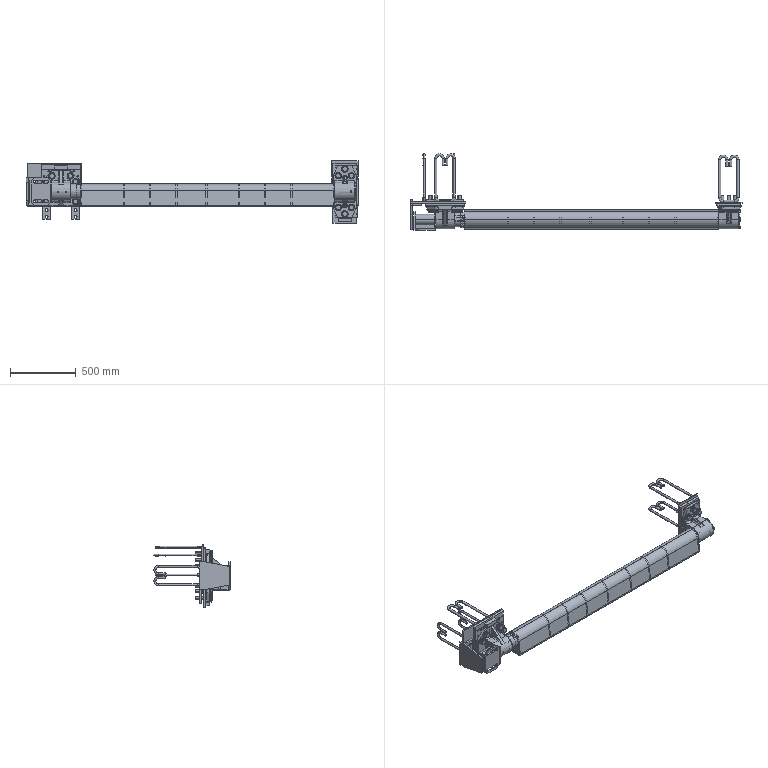Part | SolidWorks | features ReferencePattern 33, MirrorCompFeat 4, CompositeCurve 1, LocalCirPattern 1 | 116 solids | 1915 faces | box 2518 x 579 x 475 mm | volume 30927298 mm3 | plane 790 | cylinder 732 | cone 215 | torus 118 | sphere 48 | spline 12 | commonest cylinder face diameters 24 x66 16 x54 10 x48 17.5 x48 12 x44 20 x36